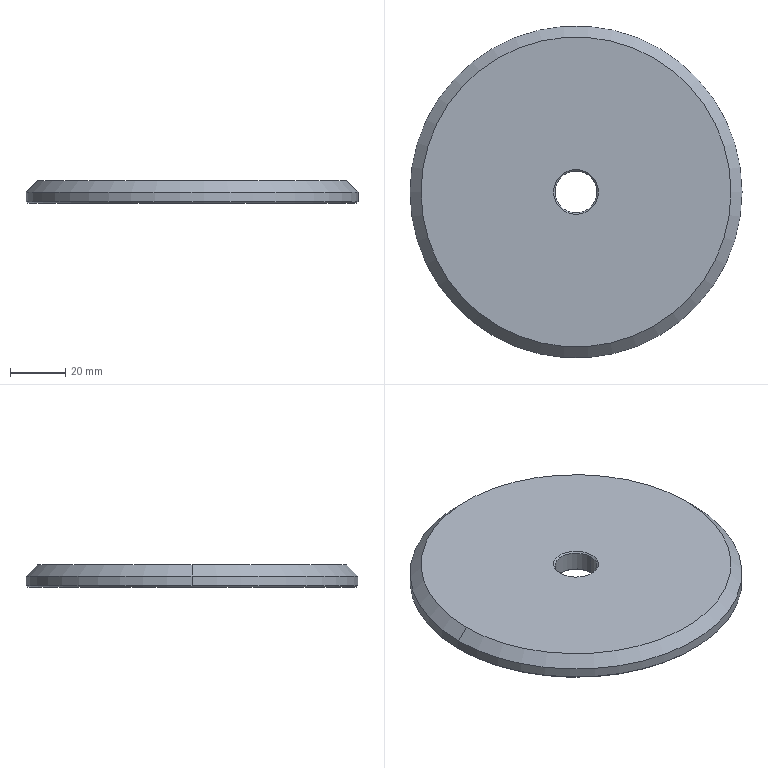Part | STEP file | 10000020576swp000-1 | 1 solid | 14 faces | box 120 x 120 x 8 mm | volume 86018 mm3 | cone 8 | cylinder 4 | plane 2 | commonest cylinder face diameters 15.2 x2 120 x2
STEP:
#1=CARTESIAN_POINT('',(-7.6,0.,7.5));
#2=VERTEX_POINT('',#1);
#3=CARTESIAN_POINT('',(7.6,0.,7.5));
#4=VERTEX_POINT('',#3);
#5=CARTESIAN_POINT('',(0.,0.,7.5));
#6=DIRECTION('',(0.,0.,1.));
#7=DIRECTION('',(1.,0.,0.));
#8=AXIS2_PLACEMENT_3D('',#5,#6,#7);
#9=CIRCLE('',#8,7.6);
#10=EDGE_CURVE('',#2,#4,#9,.T.);
#11=ORIENTED_EDGE('',*,*,#10,.F.);
#12=CARTESIAN_POINT('',(-8.1,0.,8.));
#13=VERTEX_POINT('',#12);
#14=CARTESIAN_POINT('',(-7.6,0.,7.5));
#15=DIRECTION('',(-0.7071,0.,0.7071));
#16=VECTOR('',#15,1000.);
#17=LINE('',#14,#16);
#18=EDGE_CURVE('',#2,#13,#17,.T.);
#19=ORIENTED_EDGE('',*,*,#18,.T.);
#20=CARTESIAN_POINT('',(8.1,0.,8.));
#21=VERTEX_POINT('',#20);
#22=CARTESIAN_POINT('',(0.,0.,8.));
#23=DIRECTION('',(0.,0.,-1.));
#24=DIRECTION('',(1.,0.,0.));
#25=AXIS2_PLACEMENT_3D('',#22,#23,#24);
#26=CIRCLE('',#25,8.1);
#27=EDGE_CURVE('',#21,#13,#26,.T.);
#28=ORIENTED_EDGE('',*,*,#27,.F.);
#29=CARTESIAN_POINT('',(7.6,0.,7.5));
#30=DIRECTION('',(0.7071,0.,0.7071));
#31=VECTOR('',#30,1000.);
#32=LINE('',#29,#31);
#33=EDGE_CURVE('',#4,#21,#32,.T.);
#34=ORIENTED_EDGE('',*,*,#33,.F.);
#35=EDGE_LOOP('',(#11,#19,#28,#34));
#36=FACE_OUTER_BOUND('',#35,.T.);
#37=CARTESIAN_POINT('',(0.,0.,7.5));
#38=DIRECTION('',(0.,0.,1.));
#39=DIRECTION('',(1.,0.,0.));
#40=AXIS2_PLACEMENT_3D('',#37,#38,#39);
#41=CONICAL_SURFACE('',#40,7.6,0.7854);
#42=ADVANCED_FACE('',(#36),#41,.F.);
#43=CARTESIAN_POINT('',(7.6,0.,0.5));
#44=VERTEX_POINT('',#43);
#45=CARTESIAN_POINT('',(-7.6,0.,0.5));
#46=VERTEX_POINT('',#45);
#47=CARTESIAN_POINT('',(0.,0.,0.5));
#48=DIRECTION('',(0.,0.,-1.));
#49=DIRECTION('',(1.,0.,0.));
#50=AXIS2_PLACEMENT_3D('',#47,#48,#49);
#51=CIRCLE('',#50,7.6);
#52=EDGE_CURVE('',#44,#46,#51,.T.);
#53=ORIENTED_EDGE('',*,*,#52,.F.);
#54=CARTESIAN_POINT('',(8.1,0.,0.));
#55=VERTEX_POINT('',#54);
#56=CARTESIAN_POINT('',(8.1,0.,0.));
#57=DIRECTION('',(0.7071,0.,-0.7071));
#58=VECTOR('',#57,1000.);
#59=LINE('',#56,#58);
#60=EDGE_CURVE('',#44,#55,#59,.T.);
#61=ORIENTED_EDGE('',*,*,#60,.T.);
#62=CARTESIAN_POINT('',(-8.1,0.,0.));
#63=VERTEX_POINT('',#62);
#64=CARTESIAN_POINT('',(0.,0.,0.));
#65=DIRECTION('',(0.,0.,1.));
#66=DIRECTION('',(1.,0.,0.));
#67=AXIS2_PLACEMENT_3D('',#64,#65,#66);
#68=CIRCLE('',#67,8.1);
#69=EDGE_CURVE('',#63,#55,#68,.T.);
#70=ORIENTED_EDGE('',*,*,#69,.F.);
#71=CARTESIAN_POINT('',(-8.1,0.,0.));
#72=DIRECTION('',(-0.7071,0.,-0.7071));
#73=VECTOR('',#72,1000.);
#74=LINE('',#71,#73);
#75=EDGE_CURVE('',#46,#63,#74,.T.);
#76=ORIENTED_EDGE('',*,*,#75,.F.);
#77=EDGE_LOOP('',(#53,#61,#70,#76));
#78=FACE_OUTER_BOUND('',#77,.T.);
#79=CARTESIAN_POINT('',(0.,0.,0.));
#80=DIRECTION('',(0.,0.,-1.));
#81=DIRECTION('',(-1.,0.,0.));
#82=AXIS2_PLACEMENT_3D('',#79,#80,#81);
#83=CONICAL_SURFACE('',#82,8.1,0.7854);
#84=ADVANCED_FACE('',(#78),#83,.F.);
#85=CARTESIAN_POINT('',(-59.5,0.,0.));
#86=VERTEX_POINT('',#85);
#87=CARTESIAN_POINT('',(59.5,0.,0.));
#88=VERTEX_POINT('',#87);
#89=CARTESIAN_POINT('',(0.,0.,0.));
#90=DIRECTION('',(0.,0.,-1.));
#91=DIRECTION('',(1.,0.,0.));
#92=AXIS2_PLACEMENT_3D('',#89,#90,#91);
#93=CIRCLE('',#92,59.5);
#94=EDGE_CURVE('',#86,#88,#93,.T.);
#95=ORIENTED_EDGE('',*,*,#94,.F.);
#96=CARTESIAN_POINT('',(-60.,0.,0.5));
#97=VERTEX_POINT('',#96);
#98=CARTESIAN_POINT('',(-60.,0.,0.5));
#99=DIRECTION('',(-0.7071,0.,0.7071));
#100=VECTOR('',#99,1000.);
#101=LINE('',#98,#100);
#102=EDGE_CURVE('',#86,#97,#101,.T.);
#103=ORIENTED_EDGE('',*,*,#102,.T.);
#104=CARTESIAN_POINT('',(60.,0.,0.5));
#105=VERTEX_POINT('',#104);
#106=CARTESIAN_POINT('',(0.,0.,0.5));
#107=DIRECTION('',(0.,0.,1.));
#108=DIRECTION('',(1.,0.,0.));
#109=AXIS2_PLACEMENT_3D('',#106,#107,#108);
#110=CIRCLE('',#109,60.);
#111=EDGE_CURVE('',#105,#97,#110,.T.);
#112=ORIENTED_EDGE('',*,*,#111,.F.);
#113=CARTESIAN_POINT('',(60.,0.,0.5));
#114=DIRECTION('',(0.7071,0.,0.7071));
#115=VECTOR('',#114,1000.);
#116=LINE('',#113,#115);
#117=EDGE_CURVE('',#88,#105,#116,.T.);
#118=ORIENTED_EDGE('',*,*,#117,.F.);
#119=EDGE_LOOP('',(#95,#103,#112,#118));
#120=FACE_OUTER_BOUND('',#119,.T.);
#121=CARTESIAN_POINT('',(0.,0.,0.5));
#122=DIRECTION('',(0.,0.,1.));
#123=DIRECTION('',(1.,0.,0.));
#124=AXIS2_PLACEMENT_3D('',#121,#122,#123);
#125=CONICAL_SURFACE('',#124,60.,0.7854);
#126=ADVANCED_FACE('',(#120),#125,.T.);
#127=CARTESIAN_POINT('',(56.,0.,8.));
#128=VERTEX_POINT('',#127);
#129=CARTESIAN_POINT('',(-56.,0.,8.));
#130=VERTEX_POINT('',#129);
#131=CARTESIAN_POINT('',(0.,0.,8.));
#132=DIRECTION('',(0.,0.,1.));
#133=DIRECTION('',(1.,0.,0.));
#134=AXIS2_PLACEMENT_3D('',#131,#132,#133);
#135=CIRCLE('',#134,56.);
#136=EDGE_CURVE('',#128,#130,#135,.T.);
#137=ORIENTED_EDGE('',*,*,#136,.F.);
#138=CARTESIAN_POINT('',(60.,0.,4.));
#139=VERTEX_POINT('',#138);
#140=CARTESIAN_POINT('',(56.,0.,8.));
#141=DIRECTION('',(0.7071,0.,-0.7071));
#142=VECTOR('',#141,1000.);
#143=LINE('',#140,#142);
#144=EDGE_CURVE('',#128,#139,#143,.T.);
#145=ORIENTED_EDGE('',*,*,#144,.T.);
#146=CARTESIAN_POINT('',(-60.,0.,4.));
#147=VERTEX_POINT('',#146);
#148=CARTESIAN_POINT('',(0.,0.,4.));
#149=DIRECTION('',(0.,0.,-1.));
#150=DIRECTION('',(1.,0.,0.));
#151=AXIS2_PLACEMENT_3D('',#148,#149,#150);
#152=CIRCLE('',#151,60.);
#153=EDGE_CURVE('',#147,#139,#152,.T.);
#154=ORIENTED_EDGE('',*,*,#153,.F.);
#155=CARTESIAN_POINT('',(-56.,0.,8.));
#156=DIRECTION('',(-0.7071,0.,-0.7071));
#157=VECTOR('',#156,1000.);
#158=LINE('',#155,#157);
#159=EDGE_CURVE('',#130,#147,#158,.T.);
#160=ORIENTED_EDGE('',*,*,#159,.F.);
#161=EDGE_LOOP('',(#137,#145,#154,#160));
#162=FACE_OUTER_BOUND('',#161,.T.);
#163=CARTESIAN_POINT('',(0.,0.,8.));
#164=DIRECTION('',(0.,0.,-1.));
#165=DIRECTION('',(-1.,0.,0.));
#166=AXIS2_PLACEMENT_3D('',#163,#164,#165);
#167=CONICAL_SURFACE('',#166,56.,0.7854);
#168=ADVANCED_FACE('',(#162),#167,.T.);
#169=ORIENTED_EDGE('',*,*,#10,.T.);
#170=CARTESIAN_POINT('',(7.6,0.,8.));
#171=DIRECTION('',(0.,0.,-1.));
#172=VECTOR('',#171,1000.);
#173=LINE('',#170,#172);
#174=EDGE_CURVE('',#4,#44,#173,.T.);
#175=ORIENTED_EDGE('',*,*,#174,.T.);
#176=ORIENTED_EDGE('',*,*,#52,.T.);
#177=CARTESIAN_POINT('',(-7.6,0.,8.));
#178=DIRECTION('',(0.,0.,-1.));
#179=VECTOR('',#178,1000.);
#180=LINE('',#177,#179);
#181=EDGE_CURVE('',#2,#46,#180,.T.);
#182=ORIENTED_EDGE('',*,*,#181,.F.);
#183=EDGE_LOOP('',(#169,#175,#176,#182));
#184=FACE_OUTER_BOUND('',#183,.T.);
#185=CARTESIAN_POINT('',(0.,0.,8.));
#186=DIRECTION('',(0.,0.,-1.));
#187=DIRECTION('',(-1.,0.,0.));
#188=AXIS2_PLACEMENT_3D('',#185,#186,#187);
#189=CYLINDRICAL_SURFACE('',#188,7.6);
#190=ADVANCED_FACE('',(#184),#189,.F.);
#191=ORIENTED_EDGE('',*,*,#153,.T.);
#192=CARTESIAN_POINT('',(60.,0.,8.));
#193=DIRECTION('',(0.,0.,-1.));
#194=VECTOR('',#193,1000.);
#195=LINE('',#192,#194);
#196=EDGE_CURVE('',#139,#105,#195,.T.);
#197=ORIENTED_EDGE('',*,*,#196,.T.);
#198=ORIENTED_EDGE('',*,*,#111,.T.);
#199=CARTESIAN_POINT('',(-60.,0.,8.));
#200=DIRECTION('',(0.,0.,-1.));
#201=VECTOR('',#200,1000.);
#202=LINE('',#199,#201);
#203=EDGE_CURVE('',#147,#97,#202,.T.);
#204=ORIENTED_EDGE('',*,*,#203,.F.);
#205=EDGE_LOOP('',(#191,#197,#198,#204));
#206=FACE_OUTER_BOUND('',#205,.T.);
#207=CARTESIAN_POINT('',(0.,0.,8.));
#208=DIRECTION('',(0.,0.,-1.));
#209=DIRECTION('',(-1.,0.,0.));
#210=AXIS2_PLACEMENT_3D('',#207,#208,#209);
#211=CYLINDRICAL_SURFACE('',#210,60.);
#212=ADVANCED_FACE('',(#206),#211,.T.);
#213=ORIENTED_EDGE('',*,*,#27,.T.);
#214=CARTESIAN_POINT('',(0.,0.,8.));
#215=DIRECTION('',(0.,0.,-1.));
#216=DIRECTION('',(1.,0.,0.));
#217=AXIS2_PLACEMENT_3D('',#214,#215,#216);
#218=CIRCLE('',#217,8.1);
#219=EDGE_CURVE('',#13,#21,#218,.T.);
#220=ORIENTED_EDGE('',*,*,#219,.T.);
#221=EDGE_LOOP('',(#213,#220));
#222=FACE_BOUND('',#221,.T.);
#223=CARTESIAN_POINT('',(0.,0.,8.));
#224=DIRECTION('',(0.,0.,1.));
#225=DIRECTION('',(1.,0.,0.));
#226=AXIS2_PLACEMENT_3D('',#223,#224,#225);
#227=CIRCLE('',#226,56.);
#228=EDGE_CURVE('',#130,#128,#227,.T.);
#229=ORIENTED_EDGE('',*,*,#228,.T.);
#230=ORIENTED_EDGE('',*,*,#136,.T.);
#231=EDGE_LOOP('',(#229,#230));
#232=FACE_OUTER_BOUND('',#231,.T.);
#233=CARTESIAN_POINT('',(0.,0.,8.));
#234=DIRECTION('',(0.,0.,1.));
#235=DIRECTION('',(1.,0.,0.));
#236=AXIS2_PLACEMENT_3D('',#233,#234,#235);
#237=PLANE('',#236);
#238=ADVANCED_FACE('',(#222,#232),#237,.T.);
#239=CARTESIAN_POINT('',(0.,0.,0.));
#240=DIRECTION('',(0.,0.,-1.));
#241=DIRECTION('',(1.,0.,0.));
#242=AXIS2_PLACEMENT_3D('',#239,#240,#241);
#243=CIRCLE('',#242,59.5);
#244=EDGE_CURVE('',#88,#86,#243,.T.);
#245=ORIENTED_EDGE('',*,*,#244,.T.);
#246=ORIENTED_EDGE('',*,*,#94,.T.);
#247=EDGE_LOOP('',(#245,#246));
#248=FACE_OUTER_BOUND('',#247,.T.);
#249=ORIENTED_EDGE('',*,*,#69,.T.);
#250=CARTESIAN_POINT('',(0.,0.,0.));
#251=DIRECTION('',(0.,0.,1.));
#252=DIRECTION('',(1.,0.,0.));
#253=AXIS2_PLACEMENT_3D('',#250,#251,#252);
#254=CIRCLE('',#253,8.1);
#255=EDGE_CURVE('',#55,#63,#254,.T.);
#256=ORIENTED_EDGE('',*,*,#255,.T.);
#257=EDGE_LOOP('',(#249,#256));
#258=FACE_BOUND('',#257,.T.);
#259=CARTESIAN_POINT('',(0.,0.,0.));
#260=DIRECTION('',(0.,0.,1.));
#261=DIRECTION('',(1.,0.,0.));
#262=AXIS2_PLACEMENT_3D('',#259,#260,#261);
#263=PLANE('',#262);
#264=ADVANCED_FACE('',(#248,#258),#263,.F.);
#265=ORIENTED_EDGE('',*,*,#196,.F.);
#266=CARTESIAN_POINT('',(0.,0.,4.));
#267=DIRECTION('',(0.,0.,-1.));
#268=DIRECTION('',(1.,0.,0.));
#269=AXIS2_PLACEMENT_3D('',#266,#267,#268);
#270=CIRCLE('',#269,60.);
#271=EDGE_CURVE('',#139,#147,#270,.T.);
#272=ORIENTED_EDGE('',*,*,#271,.T.);
#273=ORIENTED_EDGE('',*,*,#203,.T.);
#274=CARTESIAN_POINT('',(0.,0.,0.5));
#275=DIRECTION('',(0.,0.,1.));
#276=DIRECTION('',(1.,0.,0.));
#277=AXIS2_PLACEMENT_3D('',#274,#275,#276);
#278=CIRCLE('',#277,60.);
#279=EDGE_CURVE('',#97,#105,#278,.T.);
#280=ORIENTED_EDGE('',*,*,#279,.T.);
#281=EDGE_LOOP('',(#265,#272,#273,#280));
#282=FACE_OUTER_BOUND('',#281,.T.);
#283=CARTESIAN_POINT('',(0.,0.,8.));
#284=DIRECTION('',(0.,0.,-1.));
#285=DIRECTION('',(-1.,0.,0.));
#286=AXIS2_PLACEMENT_3D('',#283,#284,#285);
#287=CYLINDRICAL_SURFACE('',#286,60.);
#288=ADVANCED_FACE('',(#282),#287,.T.);
#289=ORIENTED_EDGE('',*,*,#174,.F.);
#290=CARTESIAN_POINT('',(0.,0.,7.5));
#291=DIRECTION('',(0.,0.,1.));
#292=DIRECTION('',(1.,0.,0.));
#293=AXIS2_PLACEMENT_3D('',#290,#291,#292);
#294=CIRCLE('',#293,7.6);
#295=EDGE_CURVE('',#4,#2,#294,.T.);
#296=ORIENTED_EDGE('',*,*,#295,.T.);
#297=ORIENTED_EDGE('',*,*,#181,.T.);
#298=CARTESIAN_POINT('',(0.,0.,0.5));
#299=DIRECTION('',(0.,0.,-1.));
#300=DIRECTION('',(1.,0.,0.));
#301=AXIS2_PLACEMENT_3D('',#298,#299,#300);
#302=CIRCLE('',#301,7.6);
#303=EDGE_CURVE('',#46,#44,#302,.T.);
#304=ORIENTED_EDGE('',*,*,#303,.T.);
#305=EDGE_LOOP('',(#289,#296,#297,#304));
#306=FACE_OUTER_BOUND('',#305,.T.);
#307=CARTESIAN_POINT('',(0.,0.,8.));
#308=DIRECTION('',(0.,0.,-1.));
#309=DIRECTION('',(-1.,0.,0.));
#310=AXIS2_PLACEMENT_3D('',#307,#308,#309);
#311=CYLINDRICAL_SURFACE('',#310,7.6);
#312=ADVANCED_FACE('',(#306),#311,.F.);
#313=ORIENTED_EDGE('',*,*,#144,.F.);
#314=ORIENTED_EDGE('',*,*,#228,.F.);
#315=ORIENTED_EDGE('',*,*,#159,.T.);
#316=ORIENTED_EDGE('',*,*,#271,.F.);
#317=EDGE_LOOP('',(#313,#314,#315,#316));
#318=FACE_OUTER_BOUND('',#317,.T.);
#319=CARTESIAN_POINT('',(0.,0.,8.));
#320=DIRECTION('',(0.,0.,-1.));
#321=DIRECTION('',(-1.,0.,0.));
#322=AXIS2_PLACEMENT_3D('',#319,#320,#321);
#323=CONICAL_SURFACE('',#322,56.,0.7854);
#324=ADVANCED_FACE('',(#318),#323,.T.);
#325=ORIENTED_EDGE('',*,*,#102,.F.);
#326=ORIENTED_EDGE('',*,*,#244,.F.);
#327=ORIENTED_EDGE('',*,*,#117,.T.);
#328=ORIENTED_EDGE('',*,*,#279,.F.);
#329=EDGE_LOOP('',(#325,#326,#327,#328));
#330=FACE_OUTER_BOUND('',#329,.T.);
#331=CARTESIAN_POINT('',(0.,0.,0.5));
#332=DIRECTION('',(0.,0.,1.));
#333=DIRECTION('',(1.,0.,0.));
#334=AXIS2_PLACEMENT_3D('',#331,#332,#333);
#335=CONICAL_SURFACE('',#334,60.,0.7854);
#336=ADVANCED_FACE('',(#330),#335,.T.);
#337=ORIENTED_EDGE('',*,*,#60,.F.);
#338=ORIENTED_EDGE('',*,*,#303,.F.);
#339=ORIENTED_EDGE('',*,*,#75,.T.);
#340=ORIENTED_EDGE('',*,*,#255,.F.);
#341=EDGE_LOOP('',(#337,#338,#339,#340));
#342=FACE_OUTER_BOUND('',#341,.T.);
#343=CARTESIAN_POINT('',(0.,0.,0.));
#344=DIRECTION('',(0.,0.,-1.));
#345=DIRECTION('',(-1.,0.,0.));
#346=AXIS2_PLACEMENT_3D('',#343,#344,#345);
#347=CONICAL_SURFACE('',#346,8.1,0.7854);
#348=ADVANCED_FACE('',(#342),#347,.F.);
#349=ORIENTED_EDGE('',*,*,#18,.F.);
#350=ORIENTED_EDGE('',*,*,#295,.F.);
#351=ORIENTED_EDGE('',*,*,#33,.T.);
#352=ORIENTED_EDGE('',*,*,#219,.F.);
#353=EDGE_LOOP('',(#349,#350,#351,#352));
#354=FACE_OUTER_BOUND('',#353,.T.);
#355=CARTESIAN_POINT('',(0.,0.,7.5));
#356=DIRECTION('',(0.,0.,1.));
#357=DIRECTION('',(1.,0.,0.));
#358=AXIS2_PLACEMENT_3D('',#355,#356,#357);
#359=CONICAL_SURFACE('',#358,7.6,0.7854);
#360=ADVANCED_FACE('',(#354),#359,.F.);
#361=CLOSED_SHELL('',(#42,#84,#126,#168,#190,#212,#238,#264,#288,#312,#324,#336,#348,#360));
#362=MANIFOLD_SOLID_BREP('',#361);
#363=CARTESIAN_POINT('',(0.,0.,0.));
#364=DIRECTION('',(0.,0.,1.));
#365=DIRECTION('',(1.,0.,0.));
#366=AXIS2_PLACEMENT_3D('',#363,#364,#365);
#367=(LENGTH_UNIT()NAMED_UNIT(*)SI_UNIT(.MILLI.,.METRE.));
#368=UNCERTAINTY_MEASURE_WITH_UNIT(LENGTH_MEASURE(0.00001),#367,'','');
#369=(NAMED_UNIT(*)PLANE_ANGLE_UNIT()SI_UNIT($,.RADIAN.));
#370=(NAMED_UNIT(*)SI_UNIT($,.STERADIAN.)SOLID_ANGLE_UNIT());
#371=(GEOMETRIC_REPRESENTATION_CONTEXT(3)GLOBAL_UNCERTAINTY_ASSIGNED_CONTEXT((#368))GLOBAL_UNIT_ASSIGNED_CONTEXT((#367,#369,#370))REPRESENTATION_CONTEXT('',''));
#372=ADVANCED_BREP_SHAPE_REPRESENTATION('',(#362,#366),#371);